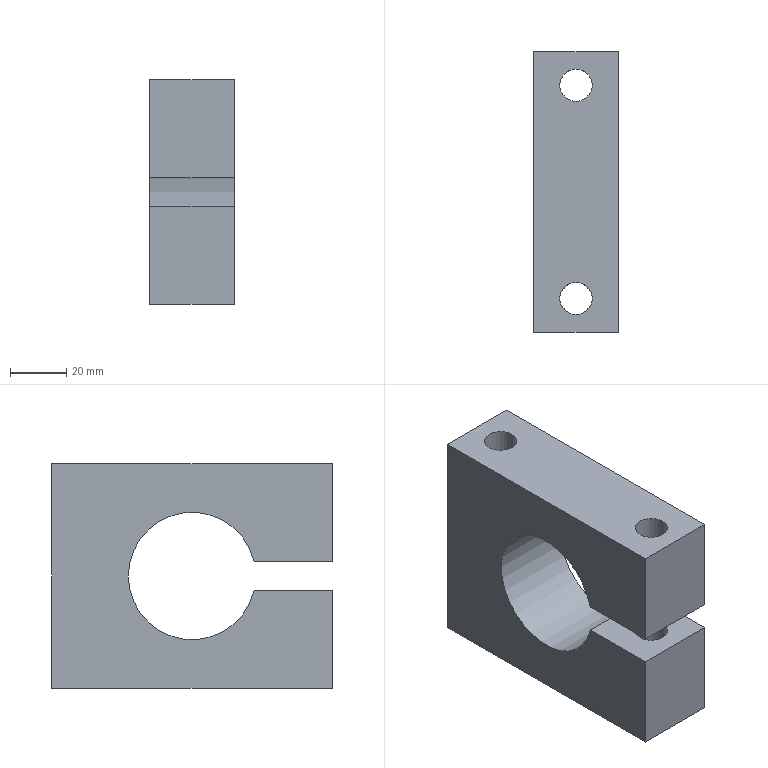Part | NX | features solid 2 | 1 solid | 17 faces | box 30 x 100 x 80 mm | volume 162111 mm3 | plane 11 | cylinder 6 | commonest cylinder face diameters 11.5 x3 16.5 x2 45.4 x1
STEP:
#1=CARTESIAN_POINT('',(-231.,-310.,165.));
#2=VERTEX_POINT('',#1);
#3=CARTESIAN_POINT('',(-201.,-310.,165.));
#4=VERTEX_POINT('',#3);
#5=CARTESIAN_POINT('',(-231.,-310.,165.));
#6=DIRECTION('',(1.,0.,0.));
#7=VECTOR('',#6,1000.);
#8=LINE('',#5,#7);
#9=EDGE_CURVE('',#2,#4,#8,.T.);
#10=ORIENTED_EDGE('',*,*,#9,.F.);
#11=CARTESIAN_POINT('',(-231.,-310.,130.));
#12=VERTEX_POINT('',#11);
#13=CARTESIAN_POINT('',(-231.,-310.,135.));
#14=DIRECTION('',(0.,0.,-1.));
#15=VECTOR('',#14,1000.);
#16=LINE('',#13,#15);
#17=EDGE_CURVE('',#2,#12,#16,.T.);
#18=ORIENTED_EDGE('',*,*,#17,.T.);
#19=CARTESIAN_POINT('',(-201.,-310.,130.));
#20=VERTEX_POINT('',#19);
#21=CARTESIAN_POINT('',(-231.,-310.,130.));
#22=DIRECTION('',(1.,0.,0.));
#23=VECTOR('',#22,1000.);
#24=LINE('',#21,#23);
#25=EDGE_CURVE('',#12,#20,#24,.T.);
#26=ORIENTED_EDGE('',*,*,#25,.T.);
#27=CARTESIAN_POINT('',(-201.,-310.,135.));
#28=DIRECTION('',(0.,0.,-1.));
#29=VECTOR('',#28,1000.);
#30=LINE('',#27,#29);
#31=EDGE_CURVE('',#4,#20,#30,.T.);
#32=ORIENTED_EDGE('',*,*,#31,.F.);
#33=EDGE_LOOP('',(#10,#18,#26,#32));
#34=FACE_BOUND('',#33,.T.);
#35=CARTESIAN_POINT('',(-231.,-310.,205.));
#36=DIRECTION('',(0.,-1.,0.));
#37=DIRECTION('',(0.,0.,1.));
#38=AXIS2_PLACEMENT_3D('',#35,#36,#37);
#39=PLANE('',#38);
#40=ADVANCED_FACE('',(#34),#39,.T.);
#41=CARTESIAN_POINT('',(-216.,-303.75,165.));
#42=VERTEX_POINT('',#41);
#43=CARTESIAN_POINT('',(-216.,-298.,165.));
#44=DIRECTION('',(0.,0.,-1.));
#45=DIRECTION('',(0.,-1.,0.));
#46=AXIS2_PLACEMENT_3D('',#43,#44,#45);
#47=CIRCLE('',#46,5.75);
#48=EDGE_CURVE('',#42,#42,#47,.F.);
#49=ORIENTED_EDGE('',*,*,#48,.T.);
#50=EDGE_LOOP('',(#49));
#51=FACE_BOUND('',#50,.T.);
#52=CARTESIAN_POINT('',(-216.,-292.25,155.));
#53=VERTEX_POINT('',#52);
#54=CARTESIAN_POINT('',(-216.,-298.,155.));
#55=DIRECTION('',(0.,0.,1.));
#56=DIRECTION('',(0.,1.,0.));
#57=AXIS2_PLACEMENT_3D('',#54,#55,#56);
#58=CIRCLE('',#57,5.75);
#59=EDGE_CURVE('',#53,#53,#58,.T.);
#60=ORIENTED_EDGE('',*,*,#59,.F.);
#61=EDGE_LOOP('',(#60));
#62=FACE_BOUND('',#61,.T.);
#63=CARTESIAN_POINT('',(-216.,-298.,230.));
#64=DIRECTION('',(0.,0.,1.));
#65=DIRECTION('',(0.,1.,0.));
#66=AXIS2_PLACEMENT_3D('',#63,#64,#65);
#67=CYLINDRICAL_SURFACE('',#66,5.75);
#68=ADVANCED_FACE('',(#51,#62),#67,.F.);
#69=ORIENTED_EDGE('',*,*,#17,.F.);
#70=CARTESIAN_POINT('',(-231.,-282.142,165.));
#71=VERTEX_POINT('',#70);
#72=CARTESIAN_POINT('',(-231.,-225.,165.));
#73=DIRECTION('',(0.,1.,0.));
#74=VECTOR('',#73,1000.);
#75=LINE('',#72,#74);
#76=EDGE_CURVE('',#2,#71,#75,.T.);
#77=ORIENTED_EDGE('',*,*,#76,.T.);
#78=CARTESIAN_POINT('',(-231.,-282.142,175.));
#79=VERTEX_POINT('',#78);
#80=CARTESIAN_POINT('',(-231.,-260.,170.));
#81=DIRECTION('',(1.,0.,0.));
#82=DIRECTION('',(0.,0.,-1.));
#83=AXIS2_PLACEMENT_3D('',#80,#81,#82);
#84=CIRCLE('',#83,22.7);
#85=EDGE_CURVE('',#79,#71,#84,.F.);
#86=ORIENTED_EDGE('',*,*,#85,.F.);
#87=CARTESIAN_POINT('',(-231.,-310.,175.));
#88=VERTEX_POINT('',#87);
#89=CARTESIAN_POINT('',(-231.,-225.,175.));
#90=DIRECTION('',(0.,1.,0.));
#91=VECTOR('',#90,1000.);
#92=LINE('',#89,#91);
#93=EDGE_CURVE('',#79,#88,#92,.F.);
#94=ORIENTED_EDGE('',*,*,#93,.T.);
#95=CARTESIAN_POINT('',(-231.,-310.,210.));
#96=VERTEX_POINT('',#95);
#97=CARTESIAN_POINT('',(-231.,-310.,135.));
#98=DIRECTION('',(0.,0.,-1.));
#99=VECTOR('',#98,1000.);
#100=LINE('',#97,#99);
#101=EDGE_CURVE('',#96,#88,#100,.T.);
#102=ORIENTED_EDGE('',*,*,#101,.F.);
#103=CARTESIAN_POINT('',(-231.,-210.,210.));
#104=VERTEX_POINT('',#103);
#105=CARTESIAN_POINT('',(-231.,-225.,210.));
#106=DIRECTION('',(0.,1.,0.));
#107=VECTOR('',#106,1000.);
#108=LINE('',#105,#107);
#109=EDGE_CURVE('',#96,#104,#108,.T.);
#110=ORIENTED_EDGE('',*,*,#109,.T.);
#111=CARTESIAN_POINT('',(-231.,-210.,130.));
#112=VERTEX_POINT('',#111);
#113=CARTESIAN_POINT('',(-231.,-210.,135.));
#114=DIRECTION('',(0.,0.,-1.));
#115=VECTOR('',#114,1000.);
#116=LINE('',#113,#115);
#117=EDGE_CURVE('',#104,#112,#116,.T.);
#118=ORIENTED_EDGE('',*,*,#117,.T.);
#119=CARTESIAN_POINT('',(-231.,-225.,130.));
#120=DIRECTION('',(0.,1.,0.));
#121=VECTOR('',#120,1000.);
#122=LINE('',#119,#121);
#123=EDGE_CURVE('',#12,#112,#122,.T.);
#124=ORIENTED_EDGE('',*,*,#123,.F.);
#125=EDGE_LOOP('',(#69,#77,#86,#94,#102,#110,#118,#124));
#126=FACE_BOUND('',#125,.T.);
#127=CARTESIAN_POINT('',(-231.,-225.,135.));
#128=DIRECTION('',(1.,0.,0.));
#129=DIRECTION('',(0.,0.,-1.));
#130=AXIS2_PLACEMENT_3D('',#127,#128,#129);
#131=PLANE('',#130);
#132=ADVANCED_FACE('',(#126),#131,.F.);
#133=CARTESIAN_POINT('',(-201.,-282.142,165.));
#134=VERTEX_POINT('',#133);
#135=CARTESIAN_POINT('',(-201.,-225.,165.));
#136=DIRECTION('',(0.,1.,0.));
#137=VECTOR('',#136,1000.);
#138=LINE('',#135,#137);
#139=EDGE_CURVE('',#4,#134,#138,.T.);
#140=ORIENTED_EDGE('',*,*,#139,.F.);
#141=ORIENTED_EDGE('',*,*,#31,.T.);
#142=CARTESIAN_POINT('',(-201.,-210.,130.));
#143=VERTEX_POINT('',#142);
#144=CARTESIAN_POINT('',(-201.,-225.,130.));
#145=DIRECTION('',(0.,1.,0.));
#146=VECTOR('',#145,1000.);
#147=LINE('',#144,#146);
#148=EDGE_CURVE('',#20,#143,#147,.T.);
#149=ORIENTED_EDGE('',*,*,#148,.T.);
#150=CARTESIAN_POINT('',(-201.,-210.,210.));
#151=VERTEX_POINT('',#150);
#152=CARTESIAN_POINT('',(-201.,-210.,135.));
#153=DIRECTION('',(0.,0.,-1.));
#154=VECTOR('',#153,1000.);
#155=LINE('',#152,#154);
#156=EDGE_CURVE('',#151,#143,#155,.T.);
#157=ORIENTED_EDGE('',*,*,#156,.F.);
#158=CARTESIAN_POINT('',(-201.,-310.,210.));
#159=VERTEX_POINT('',#158);
#160=CARTESIAN_POINT('',(-201.,-225.,210.));
#161=DIRECTION('',(0.,1.,0.));
#162=VECTOR('',#161,1000.);
#163=LINE('',#160,#162);
#164=EDGE_CURVE('',#159,#151,#163,.T.);
#165=ORIENTED_EDGE('',*,*,#164,.F.);
#166=CARTESIAN_POINT('',(-201.,-310.,175.));
#167=VERTEX_POINT('',#166);
#168=CARTESIAN_POINT('',(-201.,-310.,135.));
#169=DIRECTION('',(0.,0.,-1.));
#170=VECTOR('',#169,1000.);
#171=LINE('',#168,#170);
#172=EDGE_CURVE('',#159,#167,#171,.T.);
#173=ORIENTED_EDGE('',*,*,#172,.T.);
#174=CARTESIAN_POINT('',(-201.,-282.142,175.));
#175=VERTEX_POINT('',#174);
#176=CARTESIAN_POINT('',(-201.,-225.,175.));
#177=DIRECTION('',(0.,1.,0.));
#178=VECTOR('',#177,1000.);
#179=LINE('',#176,#178);
#180=EDGE_CURVE('',#175,#167,#179,.F.);
#181=ORIENTED_EDGE('',*,*,#180,.F.);
#182=CARTESIAN_POINT('',(-201.,-260.,170.));
#183=DIRECTION('',(1.,0.,0.));
#184=DIRECTION('',(0.,0.,-1.));
#185=AXIS2_PLACEMENT_3D('',#182,#183,#184);
#186=CIRCLE('',#185,22.7);
#187=EDGE_CURVE('',#175,#134,#186,.F.);
#188=ORIENTED_EDGE('',*,*,#187,.T.);
#189=EDGE_LOOP('',(#140,#141,#149,#157,#165,#173,#181,#188));
#190=FACE_BOUND('',#189,.T.);
#191=CARTESIAN_POINT('',(-201.,-225.,135.));
#192=DIRECTION('',(1.,0.,0.));
#193=DIRECTION('',(0.,0.,-1.));
#194=AXIS2_PLACEMENT_3D('',#191,#192,#193);
#195=PLANE('',#194);
#196=ADVANCED_FACE('',(#190),#195,.T.);
#197=ORIENTED_EDGE('',*,*,#156,.T.);
#198=CARTESIAN_POINT('',(-231.,-210.,130.));
#199=DIRECTION('',(1.,0.,0.));
#200=VECTOR('',#199,1000.);
#201=LINE('',#198,#200);
#202=EDGE_CURVE('',#112,#143,#201,.T.);
#203=ORIENTED_EDGE('',*,*,#202,.F.);
#204=ORIENTED_EDGE('',*,*,#117,.F.);
#205=CARTESIAN_POINT('',(-231.,-210.,210.));
#206=DIRECTION('',(1.,0.,0.));
#207=VECTOR('',#206,1000.);
#208=LINE('',#205,#207);
#209=EDGE_CURVE('',#104,#151,#208,.T.);
#210=ORIENTED_EDGE('',*,*,#209,.T.);
#211=EDGE_LOOP('',(#197,#203,#204,#210));
#212=FACE_BOUND('',#211,.T.);
#213=CARTESIAN_POINT('',(-231.,-210.,205.));
#214=DIRECTION('',(0.,-1.,0.));
#215=DIRECTION('',(0.,0.,1.));
#216=AXIS2_PLACEMENT_3D('',#213,#214,#215);
#217=PLANE('',#216);
#218=ADVANCED_FACE('',(#212),#217,.F.);
#219=CARTESIAN_POINT('',(-216.,-213.75,130.));
#220=VERTEX_POINT('',#219);
#221=CARTESIAN_POINT('',(-216.,-222.,130.));
#222=DIRECTION('',(0.,0.,1.));
#223=DIRECTION('',(0.,1.,0.));
#224=AXIS2_PLACEMENT_3D('',#221,#222,#223);
#225=CIRCLE('',#224,8.25);
#226=EDGE_CURVE('',#220,#220,#225,.T.);
#227=ORIENTED_EDGE('',*,*,#226,.T.);
#228=EDGE_LOOP('',(#227));
#229=FACE_BOUND('',#228,.T.);
#230=CARTESIAN_POINT('',(-216.,-289.75,130.));
#231=VERTEX_POINT('',#230);
#232=CARTESIAN_POINT('',(-216.,-298.,130.));
#233=DIRECTION('',(0.,0.,1.));
#234=DIRECTION('',(0.,1.,0.));
#235=AXIS2_PLACEMENT_3D('',#232,#233,#234);
#236=CIRCLE('',#235,8.25);
#237=EDGE_CURVE('',#231,#231,#236,.T.);
#238=ORIENTED_EDGE('',*,*,#237,.T.);
#239=EDGE_LOOP('',(#238));
#240=FACE_BOUND('',#239,.T.);
#241=ORIENTED_EDGE('',*,*,#148,.F.);
#242=ORIENTED_EDGE('',*,*,#25,.F.);
#243=ORIENTED_EDGE('',*,*,#123,.T.);
#244=ORIENTED_EDGE('',*,*,#202,.T.);
#245=EDGE_LOOP('',(#241,#242,#243,#244));
#246=FACE_BOUND('',#245,.T.);
#247=CARTESIAN_POINT('',(-231.,-295.,130.));
#248=DIRECTION('',(0.,0.,-1.));
#249=DIRECTION('',(0.,-1.,0.));
#250=AXIS2_PLACEMENT_3D('',#247,#248,#249);
#251=PLANE('',#250);
#252=ADVANCED_FACE('',(#229,#240,#246),#251,.T.);
#253=CARTESIAN_POINT('',(-231.,-310.,175.));
#254=DIRECTION('',(1.,0.,0.));
#255=VECTOR('',#254,1000.);
#256=LINE('',#253,#255);
#257=EDGE_CURVE('',#167,#88,#256,.F.);
#258=ORIENTED_EDGE('',*,*,#257,.F.);
#259=ORIENTED_EDGE('',*,*,#172,.F.);
#260=CARTESIAN_POINT('',(-231.,-310.,210.));
#261=DIRECTION('',(1.,0.,0.));
#262=VECTOR('',#261,1000.);
#263=LINE('',#260,#262);
#264=EDGE_CURVE('',#96,#159,#263,.T.);
#265=ORIENTED_EDGE('',*,*,#264,.F.);
#266=ORIENTED_EDGE('',*,*,#101,.T.);
#267=EDGE_LOOP('',(#258,#259,#265,#266));
#268=FACE_BOUND('',#267,.T.);
#269=CARTESIAN_POINT('',(-231.,-310.,205.));
#270=DIRECTION('',(0.,-1.,0.));
#271=DIRECTION('',(0.,0.,1.));
#272=AXIS2_PLACEMENT_3D('',#269,#270,#271);
#273=PLANE('',#272);
#274=ADVANCED_FACE('',(#268),#273,.T.);
#275=CARTESIAN_POINT('',(-216.,-227.75,210.));
#276=VERTEX_POINT('',#275);
#277=CARTESIAN_POINT('',(-216.,-222.,210.));
#278=DIRECTION('',(0.,0.,-1.));
#279=DIRECTION('',(0.,-1.,0.));
#280=AXIS2_PLACEMENT_3D('',#277,#278,#279);
#281=CIRCLE('',#280,5.75);
#282=EDGE_CURVE('',#276,#276,#281,.T.);
#283=ORIENTED_EDGE('',*,*,#282,.T.);
#284=EDGE_LOOP('',(#283));
#285=FACE_BOUND('',#284,.T.);
#286=CARTESIAN_POINT('',(-216.,-303.75,210.));
#287=VERTEX_POINT('',#286);
#288=CARTESIAN_POINT('',(-216.,-298.,210.));
#289=DIRECTION('',(0.,0.,-1.));
#290=DIRECTION('',(0.,-1.,0.));
#291=AXIS2_PLACEMENT_3D('',#288,#289,#290);
#292=CIRCLE('',#291,5.75);
#293=EDGE_CURVE('',#287,#287,#292,.T.);
#294=ORIENTED_EDGE('',*,*,#293,.T.);
#295=EDGE_LOOP('',(#294));
#296=FACE_BOUND('',#295,.T.);
#297=ORIENTED_EDGE('',*,*,#164,.T.);
#298=ORIENTED_EDGE('',*,*,#209,.F.);
#299=ORIENTED_EDGE('',*,*,#109,.F.);
#300=ORIENTED_EDGE('',*,*,#264,.T.);
#301=EDGE_LOOP('',(#297,#298,#299,#300));
#302=FACE_BOUND('',#301,.T.);
#303=CARTESIAN_POINT('',(-231.,-295.,210.));
#304=DIRECTION('',(0.,0.,-1.));
#305=DIRECTION('',(0.,-1.,0.));
#306=AXIS2_PLACEMENT_3D('',#303,#304,#305);
#307=PLANE('',#306);
#308=ADVANCED_FACE('',(#285,#296,#302),#307,.F.);
#309=CARTESIAN_POINT('',(-216.,-303.75,175.));
#310=VERTEX_POINT('',#309);
#311=CARTESIAN_POINT('',(-216.,-298.,175.));
#312=DIRECTION('',(0.,0.,-1.));
#313=DIRECTION('',(0.,-1.,0.));
#314=AXIS2_PLACEMENT_3D('',#311,#312,#313);
#315=CIRCLE('',#314,5.75);
#316=EDGE_CURVE('',#310,#310,#315,.T.);
#317=ORIENTED_EDGE('',*,*,#316,.T.);
#318=EDGE_LOOP('',(#317));
#319=FACE_BOUND('',#318,.T.);
#320=ORIENTED_EDGE('',*,*,#293,.F.);
#321=EDGE_LOOP('',(#320));
#322=FACE_BOUND('',#321,.T.);
#323=CARTESIAN_POINT('',(-216.,-298.,230.));
#324=DIRECTION('',(0.,0.,1.));
#325=DIRECTION('',(0.,1.,0.));
#326=AXIS2_PLACEMENT_3D('',#323,#324,#325);
#327=CYLINDRICAL_SURFACE('',#326,5.75);
#328=ADVANCED_FACE('',(#319,#322),#327,.F.);
#329=ORIENTED_EDGE('',*,*,#59,.T.);
#330=EDGE_LOOP('',(#329));
#331=FACE_BOUND('',#330,.T.);
#332=CARTESIAN_POINT('',(-216.,-289.75,155.));
#333=VERTEX_POINT('',#332);
#334=CARTESIAN_POINT('',(-216.,-298.,155.));
#335=DIRECTION('',(0.,0.,1.));
#336=DIRECTION('',(0.,1.,0.));
#337=AXIS2_PLACEMENT_3D('',#334,#335,#336);
#338=CIRCLE('',#337,8.25);
#339=EDGE_CURVE('',#333,#333,#338,.T.);
#340=ORIENTED_EDGE('',*,*,#339,.F.);
#341=EDGE_LOOP('',(#340));
#342=FACE_BOUND('',#341,.T.);
#343=CARTESIAN_POINT('',(-216.,-298.,155.));
#344=DIRECTION('',(0.,0.,1.));
#345=DIRECTION('',(0.,1.,0.));
#346=AXIS2_PLACEMENT_3D('',#343,#344,#345);
#347=PLANE('',#346);
#348=ADVANCED_FACE('',(#331,#342),#347,.F.);
#349=ORIENTED_EDGE('',*,*,#339,.T.);
#350=EDGE_LOOP('',(#349));
#351=FACE_BOUND('',#350,.T.);
#352=ORIENTED_EDGE('',*,*,#237,.F.);
#353=EDGE_LOOP('',(#352));
#354=FACE_BOUND('',#353,.T.);
#355=CARTESIAN_POINT('',(-216.,-298.,130.));
#356=DIRECTION('',(0.,0.,1.));
#357=DIRECTION('',(0.,1.,0.));
#358=AXIS2_PLACEMENT_3D('',#355,#356,#357);
#359=CYLINDRICAL_SURFACE('',#358,8.25);
#360=ADVANCED_FACE('',(#351,#354),#359,.F.);
#361=CARTESIAN_POINT('',(-216.,-216.25,155.));
#362=VERTEX_POINT('',#361);
#363=CARTESIAN_POINT('',(-216.,-222.,155.));
#364=DIRECTION('',(0.,0.,1.));
#365=DIRECTION('',(0.,1.,0.));
#366=AXIS2_PLACEMENT_3D('',#363,#364,#365);
#367=CIRCLE('',#366,5.75);
#368=EDGE_CURVE('',#362,#362,#367,.T.);
#369=ORIENTED_EDGE('',*,*,#368,.F.);
#370=EDGE_LOOP('',(#369));
#371=FACE_BOUND('',#370,.T.);
#372=ORIENTED_EDGE('',*,*,#282,.F.);
#373=EDGE_LOOP('',(#372));
#374=FACE_BOUND('',#373,.T.);
#375=CARTESIAN_POINT('',(-216.,-222.,230.));
#376=DIRECTION('',(0.,0.,1.));
#377=DIRECTION('',(0.,1.,0.));
#378=AXIS2_PLACEMENT_3D('',#375,#376,#377);
#379=CYLINDRICAL_SURFACE('',#378,5.75);
#380=ADVANCED_FACE('',(#371,#374),#379,.F.);
#381=ORIENTED_EDGE('',*,*,#368,.T.);
#382=EDGE_LOOP('',(#381));
#383=FACE_BOUND('',#382,.T.);
#384=CARTESIAN_POINT('',(-216.,-213.75,155.));
#385=VERTEX_POINT('',#384);
#386=CARTESIAN_POINT('',(-216.,-222.,155.));
#387=DIRECTION('',(0.,0.,1.));
#388=DIRECTION('',(0.,1.,0.));
#389=AXIS2_PLACEMENT_3D('',#386,#387,#388);
#390=CIRCLE('',#389,8.25);
#391=EDGE_CURVE('',#385,#385,#390,.T.);
#392=ORIENTED_EDGE('',*,*,#391,.F.);
#393=EDGE_LOOP('',(#392));
#394=FACE_BOUND('',#393,.T.);
#395=CARTESIAN_POINT('',(-216.,-222.,155.));
#396=DIRECTION('',(0.,0.,1.));
#397=DIRECTION('',(0.,1.,0.));
#398=AXIS2_PLACEMENT_3D('',#395,#396,#397);
#399=PLANE('',#398);
#400=ADVANCED_FACE('',(#383,#394),#399,.F.);
#401=ORIENTED_EDGE('',*,*,#391,.T.);
#402=EDGE_LOOP('',(#401));
#403=FACE_BOUND('',#402,.T.);
#404=ORIENTED_EDGE('',*,*,#226,.F.);
#405=EDGE_LOOP('',(#404));
#406=FACE_BOUND('',#405,.T.);
#407=CARTESIAN_POINT('',(-216.,-222.,130.));
#408=DIRECTION('',(0.,0.,1.));
#409=DIRECTION('',(0.,1.,0.));
#410=AXIS2_PLACEMENT_3D('',#407,#408,#409);
#411=CYLINDRICAL_SURFACE('',#410,8.25);
#412=ADVANCED_FACE('',(#403,#406),#411,.F.);
#413=CARTESIAN_POINT('',(54.,-282.142,165.));
#414=DIRECTION('',(-1.,0.,0.));
#415=VECTOR('',#414,1000.);
#416=LINE('',#413,#415);
#417=EDGE_CURVE('',#134,#71,#416,.T.);
#418=ORIENTED_EDGE('',*,*,#417,.F.);
#419=ORIENTED_EDGE('',*,*,#187,.F.);
#420=CARTESIAN_POINT('',(54.,-282.142,175.));
#421=DIRECTION('',(-1.,0.,0.));
#422=VECTOR('',#421,1000.);
#423=LINE('',#420,#422);
#424=EDGE_CURVE('',#79,#175,#423,.F.);
#425=ORIENTED_EDGE('',*,*,#424,.F.);
#426=ORIENTED_EDGE('',*,*,#85,.T.);
#427=EDGE_LOOP('',(#418,#419,#425,#426));
#428=FACE_BOUND('',#427,.T.);
#429=CARTESIAN_POINT('',(54.,-260.,170.));
#430=DIRECTION('',(-1.,0.,0.));
#431=DIRECTION('',(0.,0.,1.));
#432=AXIS2_PLACEMENT_3D('',#429,#430,#431);
#433=CYLINDRICAL_SURFACE('',#432,22.7);
#434=ADVANCED_FACE('',(#428),#433,.F.);
#435=ORIENTED_EDGE('',*,*,#257,.T.);
#436=ORIENTED_EDGE('',*,*,#93,.F.);
#437=ORIENTED_EDGE('',*,*,#424,.T.);
#438=ORIENTED_EDGE('',*,*,#180,.T.);
#439=EDGE_LOOP('',(#435,#436,#437,#438));
#440=FACE_BOUND('',#439,.T.);
#441=ORIENTED_EDGE('',*,*,#316,.F.);
#442=EDGE_LOOP('',(#441));
#443=FACE_BOUND('',#442,.T.);
#444=CARTESIAN_POINT('',(-201.,-410.,175.));
#445=DIRECTION('',(0.,0.,-1.));
#446=DIRECTION('',(0.,1.,0.));
#447=AXIS2_PLACEMENT_3D('',#444,#445,#446);
#448=PLANE('',#447);
#449=ADVANCED_FACE('',(#440,#443),#448,.T.);
#450=ORIENTED_EDGE('',*,*,#9,.T.);
#451=ORIENTED_EDGE('',*,*,#139,.T.);
#452=ORIENTED_EDGE('',*,*,#417,.T.);
#453=ORIENTED_EDGE('',*,*,#76,.F.);
#454=EDGE_LOOP('',(#450,#451,#452,#453));
#455=FACE_BOUND('',#454,.T.);
#456=ORIENTED_EDGE('',*,*,#48,.F.);
#457=EDGE_LOOP('',(#456));
#458=FACE_BOUND('',#457,.T.);
#459=CARTESIAN_POINT('',(-201.,-410.,165.));
#460=DIRECTION('',(0.,0.,-1.));
#461=DIRECTION('',(0.,1.,0.));
#462=AXIS2_PLACEMENT_3D('',#459,#460,#461);
#463=PLANE('',#462);
#464=ADVANCED_FACE('',(#455,#458),#463,.F.);
#465=CLOSED_SHELL('',(#40,#68,#132,#196,#218,#252,#274,#308,#328,#348,#360,#380,#400,#412,#434,#449,#464));
#466=MANIFOLD_SOLID_BREP('',#465);
#467=(LENGTH_UNIT()NAMED_UNIT(*)SI_UNIT(.MILLI.,.METRE.));
#468=UNCERTAINTY_MEASURE_WITH_UNIT(LENGTH_MEASURE(0.00001),#467,'','');
#469=(NAMED_UNIT(*)PLANE_ANGLE_UNIT()SI_UNIT($,.RADIAN.));
#470=(NAMED_UNIT(*)SI_UNIT($,.STERADIAN.)SOLID_ANGLE_UNIT());
#471=(GEOMETRIC_REPRESENTATION_CONTEXT(3)GLOBAL_UNCERTAINTY_ASSIGNED_CONTEXT((#468))GLOBAL_UNIT_ASSIGNED_CONTEXT((#467,#469,#470))REPRESENTATION_CONTEXT('',''));
#472=ADVANCED_BREP_SHAPE_REPRESENTATION('',(#466),#471);